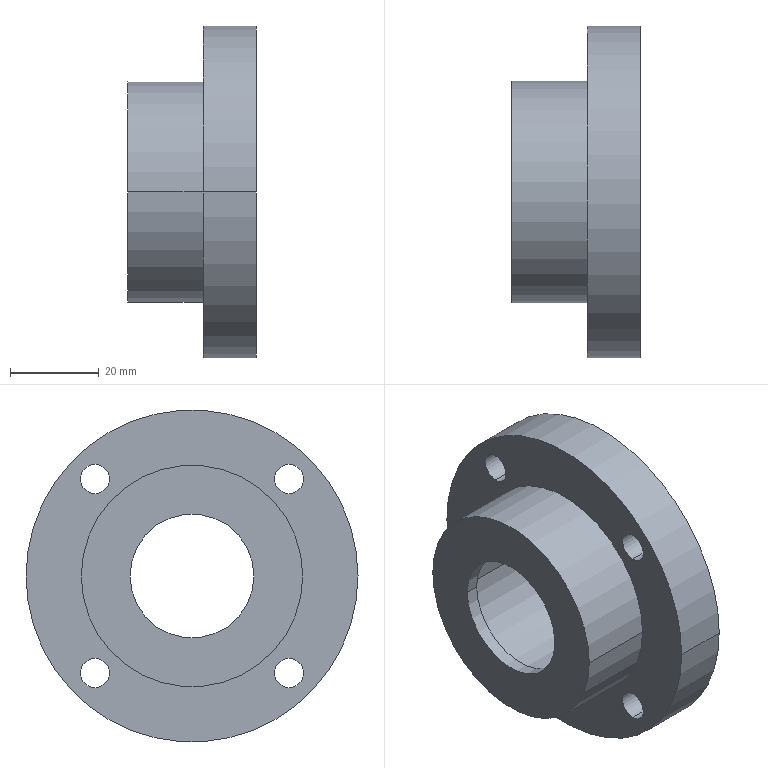Part | SolidWorks | features HoleWzd 2, Chamfer 1, Revolution 1 | 1 solid | 53 faces | box 29 x 75 x 75 mm | volume 54196 mm3 | cylinder 34 | cone 10 | plane 9 | commonest cylinder face diameters 2.5 x8 6.6 x8 11 x8 28 x2 32 x2 48 x2
STEP:
#1=CARTESIAN_POINT('',(-6.5,-16.,0.));
#2=VERTEX_POINT('',#1);
#3=CARTESIAN_POINT('',(-6.5,16.,0.));
#4=VERTEX_POINT('',#3);
#5=CARTESIAN_POINT('',(-6.5,0.,0.));
#6=DIRECTION('',(1.,0.,0.));
#7=DIRECTION('',(0.,1.,0.));
#8=AXIS2_PLACEMENT_3D('',#5,#6,#7);
#9=CIRCLE('',#8,16.);
#10=EDGE_CURVE('',#2,#4,#9,.T.);
#11=ORIENTED_EDGE('',*,*,#10,.F.);
#12=CARTESIAN_POINT('',(-6.,-16.5,0.));
#13=VERTEX_POINT('',#12);
#14=CARTESIAN_POINT('',(-6.5,-16.,0.));
#15=DIRECTION('',(0.7071,-0.7071,0.));
#16=VECTOR('',#15,1000.);
#17=LINE('',#14,#16);
#18=EDGE_CURVE('',#2,#13,#17,.T.);
#19=ORIENTED_EDGE('',*,*,#18,.T.);
#20=CARTESIAN_POINT('',(-6.,16.5,0.));
#21=VERTEX_POINT('',#20);
#22=CARTESIAN_POINT('',(-6.,0.,0.));
#23=DIRECTION('',(-1.,0.,0.));
#24=DIRECTION('',(0.,1.,0.));
#25=AXIS2_PLACEMENT_3D('',#22,#23,#24);
#26=CIRCLE('',#25,16.5);
#27=EDGE_CURVE('',#21,#13,#26,.T.);
#28=ORIENTED_EDGE('',*,*,#27,.F.);
#29=CARTESIAN_POINT('',(-6.5,16.,0.));
#30=DIRECTION('',(0.7071,0.7071,0.));
#31=VECTOR('',#30,1000.);
#32=LINE('',#29,#31);
#33=EDGE_CURVE('',#4,#21,#32,.T.);
#34=ORIENTED_EDGE('',*,*,#33,.F.);
#35=EDGE_LOOP('',(#11,#19,#28,#34));
#36=FACE_OUTER_BOUND('',#35,.T.);
#37=CARTESIAN_POINT('',(-6.5,0.,0.));
#38=DIRECTION('',(1.,0.,0.));
#39=DIRECTION('',(0.,1.,0.));
#40=AXIS2_PLACEMENT_3D('',#37,#38,#39);
#41=CONICAL_SURFACE('',#40,16.,0.7854);
#42=ADVANCED_FACE('',(#36),#41,.F.);
#43=CARTESIAN_POINT('',(-14.5,20.,1.25));
#44=VERTEX_POINT('',#43);
#45=CARTESIAN_POINT('',(-14.5,20.,-1.25));
#46=VERTEX_POINT('',#45);
#47=CARTESIAN_POINT('',(-14.5,20.,0.));
#48=DIRECTION('',(1.,0.,0.));
#49=DIRECTION('',(0.,0.,-1.));
#50=AXIS2_PLACEMENT_3D('',#47,#48,#49);
#51=CIRCLE('',#50,1.25);
#52=EDGE_CURVE('',#44,#46,#51,.T.);
#53=ORIENTED_EDGE('',*,*,#52,.F.);
#54=CARTESIAN_POINT('',(-6.,20.,1.25));
#55=VERTEX_POINT('',#54);
#56=CARTESIAN_POINT('',(-6.,20.,1.25));
#57=DIRECTION('',(1.,0.,0.));
#58=VECTOR('',#57,1000.);
#59=LINE('',#56,#58);
#60=EDGE_CURVE('',#44,#55,#59,.T.);
#61=ORIENTED_EDGE('',*,*,#60,.T.);
#62=CARTESIAN_POINT('',(-6.,20.,-1.25));
#63=VERTEX_POINT('',#62);
#64=CARTESIAN_POINT('',(-6.,20.,0.));
#65=DIRECTION('',(1.,0.,0.));
#66=DIRECTION('',(0.,0.,-1.));
#67=AXIS2_PLACEMENT_3D('',#64,#65,#66);
#68=CIRCLE('',#67,1.25);
#69=EDGE_CURVE('',#55,#63,#68,.T.);
#70=ORIENTED_EDGE('',*,*,#69,.T.);
#71=CARTESIAN_POINT('',(-6.,20.,-1.25));
#72=DIRECTION('',(1.,0.,0.));
#73=VECTOR('',#72,1000.);
#74=LINE('',#71,#73);
#75=EDGE_CURVE('',#46,#63,#74,.T.);
#76=ORIENTED_EDGE('',*,*,#75,.F.);
#77=EDGE_LOOP('',(#53,#61,#70,#76));
#78=FACE_OUTER_BOUND('',#77,.T.);
#79=CARTESIAN_POINT('',(-6.,20.,0.));
#80=DIRECTION('',(1.,0.,0.));
#81=DIRECTION('',(0.,0.,-1.));
#82=AXIS2_PLACEMENT_3D('',#79,#80,#81);
#83=CYLINDRICAL_SURFACE('',#82,1.25);
#84=ADVANCED_FACE('',(#78),#83,.F.);
#85=CARTESIAN_POINT('',(-15.251,20.,0.));
#86=VERTEX_POINT('',#85);
#87=CARTESIAN_POINT('',(-14.5,20.,-1.25));
#88=DIRECTION('',(0.515,0.,-0.8572));
#89=VECTOR('',#88,1000.);
#90=LINE('',#87,#89);
#91=EDGE_CURVE('',#86,#46,#90,.T.);
#92=ORIENTED_EDGE('',*,*,#91,.F.);
#93=CARTESIAN_POINT('',(-14.5,20.,1.25));
#94=DIRECTION('',(0.515,0.,0.8572));
#95=VECTOR('',#94,1000.);
#96=LINE('',#93,#95);
#97=EDGE_CURVE('',#86,#44,#96,.T.);
#98=ORIENTED_EDGE('',*,*,#97,.T.);
#99=ORIENTED_EDGE('',*,*,#52,.T.);
#100=EDGE_LOOP('',(#92,#98,#99));
#101=FACE_OUTER_BOUND('',#100,.T.);
#102=CARTESIAN_POINT('',(-14.5,20.,0.));
#103=DIRECTION('',(1.,0.,0.));
#104=DIRECTION('',(0.,0.,-1.));
#105=AXIS2_PLACEMENT_3D('',#102,#103,#104);
#106=CONICAL_SURFACE('',#105,1.25,1.03);
#107=ADVANCED_FACE('',(#101),#106,.F.);
#108=CARTESIAN_POINT('',(-14.5,0.,21.25));
#109=VERTEX_POINT('',#108);
#110=CARTESIAN_POINT('',(-14.5,0.,18.75));
#111=VERTEX_POINT('',#110);
#112=CARTESIAN_POINT('',(-14.5,0.,20.));
#113=DIRECTION('',(1.,0.,0.));
#114=DIRECTION('',(0.,0.,-1.));
#115=AXIS2_PLACEMENT_3D('',#112,#113,#114);
#116=CIRCLE('',#115,1.25);
#117=EDGE_CURVE('',#109,#111,#116,.T.);
#118=ORIENTED_EDGE('',*,*,#117,.F.);
#119=CARTESIAN_POINT('',(-6.,0.,21.25));
#120=VERTEX_POINT('',#119);
#121=CARTESIAN_POINT('',(-6.,0.,21.25));
#122=DIRECTION('',(1.,0.,0.));
#123=VECTOR('',#122,1000.);
#124=LINE('',#121,#123);
#125=EDGE_CURVE('',#109,#120,#124,.T.);
#126=ORIENTED_EDGE('',*,*,#125,.T.);
#127=CARTESIAN_POINT('',(-6.,0.,18.75));
#128=VERTEX_POINT('',#127);
#129=CARTESIAN_POINT('',(-6.,0.,20.));
#130=DIRECTION('',(1.,0.,0.));
#131=DIRECTION('',(0.,0.,-1.));
#132=AXIS2_PLACEMENT_3D('',#129,#130,#131);
#133=CIRCLE('',#132,1.25);
#134=EDGE_CURVE('',#120,#128,#133,.T.);
#135=ORIENTED_EDGE('',*,*,#134,.T.);
#136=CARTESIAN_POINT('',(-6.,0.,18.75));
#137=DIRECTION('',(1.,0.,0.));
#138=VECTOR('',#137,1000.);
#139=LINE('',#136,#138);
#140=EDGE_CURVE('',#111,#128,#139,.T.);
#141=ORIENTED_EDGE('',*,*,#140,.F.);
#142=EDGE_LOOP('',(#118,#126,#135,#141));
#143=FACE_OUTER_BOUND('',#142,.T.);
#144=CARTESIAN_POINT('',(-6.,0.,20.));
#145=DIRECTION('',(1.,0.,0.));
#146=DIRECTION('',(0.,0.,-1.));
#147=AXIS2_PLACEMENT_3D('',#144,#145,#146);
#148=CYLINDRICAL_SURFACE('',#147,1.25);
#149=ADVANCED_FACE('',(#143),#148,.F.);
#150=CARTESIAN_POINT('',(-15.251,0.,20.));
#151=VERTEX_POINT('',#150);
#152=CARTESIAN_POINT('',(-14.5,0.,18.75));
#153=DIRECTION('',(0.515,0.,-0.8572));
#154=VECTOR('',#153,1000.);
#155=LINE('',#152,#154);
#156=EDGE_CURVE('',#151,#111,#155,.T.);
#157=ORIENTED_EDGE('',*,*,#156,.F.);
#158=CARTESIAN_POINT('',(-14.5,0.,21.25));
#159=DIRECTION('',(0.515,0.,0.8572));
#160=VECTOR('',#159,1000.);
#161=LINE('',#158,#160);
#162=EDGE_CURVE('',#151,#109,#161,.T.);
#163=ORIENTED_EDGE('',*,*,#162,.T.);
#164=ORIENTED_EDGE('',*,*,#117,.T.);
#165=EDGE_LOOP('',(#157,#163,#164));
#166=FACE_OUTER_BOUND('',#165,.T.);
#167=CARTESIAN_POINT('',(-14.5,0.,20.));
#168=DIRECTION('',(1.,0.,0.));
#169=DIRECTION('',(0.,0.,-1.));
#170=AXIS2_PLACEMENT_3D('',#167,#168,#169);
#171=CONICAL_SURFACE('',#170,1.25,1.03);
#172=ADVANCED_FACE('',(#166),#171,.F.);
#173=CARTESIAN_POINT('',(-14.5,-20.,1.25));
#174=VERTEX_POINT('',#173);
#175=CARTESIAN_POINT('',(-14.5,-20.,-1.25));
#176=VERTEX_POINT('',#175);
#177=CARTESIAN_POINT('',(-14.5,-20.,0.));
#178=DIRECTION('',(1.,0.,0.));
#179=DIRECTION('',(0.,0.,-1.));
#180=AXIS2_PLACEMENT_3D('',#177,#178,#179);
#181=CIRCLE('',#180,1.25);
#182=EDGE_CURVE('',#174,#176,#181,.T.);
#183=ORIENTED_EDGE('',*,*,#182,.F.);
#184=CARTESIAN_POINT('',(-6.,-20.,1.25));
#185=VERTEX_POINT('',#184);
#186=CARTESIAN_POINT('',(-6.,-20.,1.25));
#187=DIRECTION('',(1.,0.,0.));
#188=VECTOR('',#187,1000.);
#189=LINE('',#186,#188);
#190=EDGE_CURVE('',#174,#185,#189,.T.);
#191=ORIENTED_EDGE('',*,*,#190,.T.);
#192=CARTESIAN_POINT('',(-6.,-20.,-1.25));
#193=VERTEX_POINT('',#192);
#194=CARTESIAN_POINT('',(-6.,-20.,0.));
#195=DIRECTION('',(1.,0.,0.));
#196=DIRECTION('',(0.,0.,-1.));
#197=AXIS2_PLACEMENT_3D('',#194,#195,#196);
#198=CIRCLE('',#197,1.25);
#199=EDGE_CURVE('',#185,#193,#198,.T.);
#200=ORIENTED_EDGE('',*,*,#199,.T.);
#201=CARTESIAN_POINT('',(-6.,-20.,-1.25));
#202=DIRECTION('',(1.,0.,0.));
#203=VECTOR('',#202,1000.);
#204=LINE('',#201,#203);
#205=EDGE_CURVE('',#176,#193,#204,.T.);
#206=ORIENTED_EDGE('',*,*,#205,.F.);
#207=EDGE_LOOP('',(#183,#191,#200,#206));
#208=FACE_OUTER_BOUND('',#207,.T.);
#209=CARTESIAN_POINT('',(-6.,-20.,0.));
#210=DIRECTION('',(1.,0.,0.));
#211=DIRECTION('',(0.,0.,-1.));
#212=AXIS2_PLACEMENT_3D('',#209,#210,#211);
#213=CYLINDRICAL_SURFACE('',#212,1.25);
#214=ADVANCED_FACE('',(#208),#213,.F.);
#215=CARTESIAN_POINT('',(-15.251,-20.,0.));
#216=VERTEX_POINT('',#215);
#217=CARTESIAN_POINT('',(-14.5,-20.,-1.25));
#218=DIRECTION('',(0.515,0.,-0.8572));
#219=VECTOR('',#218,1000.);
#220=LINE('',#217,#219);
#221=EDGE_CURVE('',#216,#176,#220,.T.);
#222=ORIENTED_EDGE('',*,*,#221,.F.);
#223=CARTESIAN_POINT('',(-14.5,-20.,1.25));
#224=DIRECTION('',(0.515,0.,0.8572));
#225=VECTOR('',#224,1000.);
#226=LINE('',#223,#225);
#227=EDGE_CURVE('',#216,#174,#226,.T.);
#228=ORIENTED_EDGE('',*,*,#227,.T.);
#229=ORIENTED_EDGE('',*,*,#182,.T.);
#230=EDGE_LOOP('',(#222,#228,#229));
#231=FACE_OUTER_BOUND('',#230,.T.);
#232=CARTESIAN_POINT('',(-14.5,-20.,0.));
#233=DIRECTION('',(1.,0.,0.));
#234=DIRECTION('',(0.,0.,-1.));
#235=AXIS2_PLACEMENT_3D('',#232,#233,#234);
#236=CONICAL_SURFACE('',#235,1.25,1.03);
#237=ADVANCED_FACE('',(#231),#236,.F.);
#238=CARTESIAN_POINT('',(-14.5,0.,-18.75));
#239=VERTEX_POINT('',#238);
#240=CARTESIAN_POINT('',(-14.5,0.,-21.25));
#241=VERTEX_POINT('',#240);
#242=CARTESIAN_POINT('',(-14.5,0.,-20.));
#243=DIRECTION('',(1.,0.,0.));
#244=DIRECTION('',(0.,0.,-1.));
#245=AXIS2_PLACEMENT_3D('',#242,#243,#244);
#246=CIRCLE('',#245,1.25);
#247=EDGE_CURVE('',#239,#241,#246,.T.);
#248=ORIENTED_EDGE('',*,*,#247,.F.);
#249=CARTESIAN_POINT('',(-6.,0.,-18.75));
#250=VERTEX_POINT('',#249);
#251=CARTESIAN_POINT('',(-6.,0.,-18.75));
#252=DIRECTION('',(1.,0.,0.));
#253=VECTOR('',#252,1000.);
#254=LINE('',#251,#253);
#255=EDGE_CURVE('',#239,#250,#254,.T.);
#256=ORIENTED_EDGE('',*,*,#255,.T.);
#257=CARTESIAN_POINT('',(-6.,0.,-21.25));
#258=VERTEX_POINT('',#257);
#259=CARTESIAN_POINT('',(-6.,0.,-20.));
#260=DIRECTION('',(1.,0.,0.));
#261=DIRECTION('',(0.,0.,-1.));
#262=AXIS2_PLACEMENT_3D('',#259,#260,#261);
#263=CIRCLE('',#262,1.25);
#264=EDGE_CURVE('',#250,#258,#263,.T.);
#265=ORIENTED_EDGE('',*,*,#264,.T.);
#266=CARTESIAN_POINT('',(-6.,0.,-21.25));
#267=DIRECTION('',(1.,0.,0.));
#268=VECTOR('',#267,1000.);
#269=LINE('',#266,#268);
#270=EDGE_CURVE('',#241,#258,#269,.T.);
#271=ORIENTED_EDGE('',*,*,#270,.F.);
#272=EDGE_LOOP('',(#248,#256,#265,#271));
#273=FACE_OUTER_BOUND('',#272,.T.);
#274=CARTESIAN_POINT('',(-6.,0.,-20.));
#275=DIRECTION('',(1.,0.,0.));
#276=DIRECTION('',(0.,0.,-1.));
#277=AXIS2_PLACEMENT_3D('',#274,#275,#276);
#278=CYLINDRICAL_SURFACE('',#277,1.25);
#279=ADVANCED_FACE('',(#273),#278,.F.);
#280=CARTESIAN_POINT('',(-15.251,0.,-20.));
#281=VERTEX_POINT('',#280);
#282=CARTESIAN_POINT('',(-14.5,0.,-21.25));
#283=DIRECTION('',(0.515,0.,-0.8572));
#284=VECTOR('',#283,1000.);
#285=LINE('',#282,#284);
#286=EDGE_CURVE('',#281,#241,#285,.T.);
#287=ORIENTED_EDGE('',*,*,#286,.F.);
#288=CARTESIAN_POINT('',(-14.5,0.,-18.75));
#289=DIRECTION('',(0.515,0.,0.8572));
#290=VECTOR('',#289,1000.);
#291=LINE('',#288,#290);
#292=EDGE_CURVE('',#281,#239,#291,.T.);
#293=ORIENTED_EDGE('',*,*,#292,.T.);
#294=ORIENTED_EDGE('',*,*,#247,.T.);
#295=EDGE_LOOP('',(#287,#293,#294));
#296=FACE_OUTER_BOUND('',#295,.T.);
#297=CARTESIAN_POINT('',(-14.5,0.,-20.));
#298=DIRECTION('',(1.,0.,0.));
#299=DIRECTION('',(0.,0.,-1.));
#300=AXIS2_PLACEMENT_3D('',#297,#298,#299);
#301=CONICAL_SURFACE('',#300,1.25,1.03);
#302=ADVANCED_FACE('',(#296),#301,.F.);
#303=CARTESIAN_POINT('',(-6.5,21.92,27.42));
#304=VERTEX_POINT('',#303);
#305=CARTESIAN_POINT('',(-6.5,21.92,16.42));
#306=VERTEX_POINT('',#305);
#307=CARTESIAN_POINT('',(-6.5,21.92,21.92));
#308=DIRECTION('',(1.,0.,0.));
#309=DIRECTION('',(0.,0.,-1.));
#310=AXIS2_PLACEMENT_3D('',#307,#308,#309);
#311=CIRCLE('',#310,5.5);
#312=EDGE_CURVE('',#304,#306,#311,.T.);
#313=ORIENTED_EDGE('',*,*,#312,.F.);
#314=CARTESIAN_POINT('',(0.,21.92,27.42));
#315=VERTEX_POINT('',#314);
#316=CARTESIAN_POINT('',(0.,21.92,27.42));
#317=DIRECTION('',(1.,0.,0.));
#318=VECTOR('',#317,1000.);
#319=LINE('',#316,#318);
#320=EDGE_CURVE('',#304,#315,#319,.T.);
#321=ORIENTED_EDGE('',*,*,#320,.T.);
#322=CARTESIAN_POINT('',(0.,21.92,16.42));
#323=VERTEX_POINT('',#322);
#324=CARTESIAN_POINT('',(0.,21.92,21.92));
#325=DIRECTION('',(1.,0.,0.));
#326=DIRECTION('',(0.,0.,-1.));
#327=AXIS2_PLACEMENT_3D('',#324,#325,#326);
#328=CIRCLE('',#327,5.5);
#329=EDGE_CURVE('',#315,#323,#328,.T.);
#330=ORIENTED_EDGE('',*,*,#329,.T.);
#331=CARTESIAN_POINT('',(0.,21.92,16.42));
#332=DIRECTION('',(1.,0.,0.));
#333=VECTOR('',#332,1000.);
#334=LINE('',#331,#333);
#335=EDGE_CURVE('',#306,#323,#334,.T.);
#336=ORIENTED_EDGE('',*,*,#335,.F.);
#337=EDGE_LOOP('',(#313,#321,#330,#336));
#338=FACE_OUTER_BOUND('',#337,.T.);
#339=CARTESIAN_POINT('',(0.,21.92,21.92));
#340=DIRECTION('',(1.,0.,0.));
#341=DIRECTION('',(0.,0.,-1.));
#342=AXIS2_PLACEMENT_3D('',#339,#340,#341);
#343=CYLINDRICAL_SURFACE('',#342,5.5);
#344=ADVANCED_FACE('',(#338),#343,.F.);
#345=CARTESIAN_POINT('',(-12.,21.92,18.62));
#346=VERTEX_POINT('',#345);
#347=CARTESIAN_POINT('',(-12.,21.92,25.22));
#348=VERTEX_POINT('',#347);
#349=CARTESIAN_POINT('',(-12.,21.92,21.92));
#350=DIRECTION('',(-1.,0.,0.));
#351=DIRECTION('',(0.,-1.,0.));
#352=AXIS2_PLACEMENT_3D('',#349,#350,#351);
#353=CIRCLE('',#352,3.3);
#354=EDGE_CURVE('',#346,#348,#353,.T.);
#355=ORIENTED_EDGE('',*,*,#354,.T.);
#356=CARTESIAN_POINT('',(-6.5,21.92,25.22));
#357=VERTEX_POINT('',#356);
#358=CARTESIAN_POINT('',(0.,21.92,25.22));
#359=DIRECTION('',(1.,0.,0.));
#360=VECTOR('',#359,1000.);
#361=LINE('',#358,#360);
#362=EDGE_CURVE('',#348,#357,#361,.T.);
#363=ORIENTED_EDGE('',*,*,#362,.T.);
#364=CARTESIAN_POINT('',(-6.5,21.92,18.62));
#365=VERTEX_POINT('',#364);
#366=CARTESIAN_POINT('',(-6.5,21.92,21.92));
#367=DIRECTION('',(1.,0.,0.));
#368=DIRECTION('',(0.,0.,-1.));
#369=AXIS2_PLACEMENT_3D('',#366,#367,#368);
#370=CIRCLE('',#369,3.3);
#371=EDGE_CURVE('',#357,#365,#370,.T.);
#372=ORIENTED_EDGE('',*,*,#371,.T.);
#373=CARTESIAN_POINT('',(0.,21.92,18.62));
#374=DIRECTION('',(1.,0.,0.));
#375=VECTOR('',#374,1000.);
#376=LINE('',#373,#375);
#377=EDGE_CURVE('',#346,#365,#376,.T.);
#378=ORIENTED_EDGE('',*,*,#377,.F.);
#379=EDGE_LOOP('',(#355,#363,#372,#378));
#380=FACE_OUTER_BOUND('',#379,.T.);
#381=CARTESIAN_POINT('',(0.,21.92,21.92));
#382=DIRECTION('',(1.,0.,0.));
#383=DIRECTION('',(0.,0.,-1.));
#384=AXIS2_PLACEMENT_3D('',#381,#382,#383);
#385=CYLINDRICAL_SURFACE('',#384,3.3);
#386=ADVANCED_FACE('',(#380),#385,.F.);
#387=CARTESIAN_POINT('',(-6.5,21.92,-16.42));
#388=VERTEX_POINT('',#387);
#389=CARTESIAN_POINT('',(-6.5,21.92,-27.42));
#390=VERTEX_POINT('',#389);
#391=CARTESIAN_POINT('',(-6.5,21.92,-21.92));
#392=DIRECTION('',(1.,0.,0.));
#393=DIRECTION('',(0.,0.,-1.));
#394=AXIS2_PLACEMENT_3D('',#391,#392,#393);
#395=CIRCLE('',#394,5.5);
#396=EDGE_CURVE('',#388,#390,#395,.T.);
#397=ORIENTED_EDGE('',*,*,#396,.F.);
#398=CARTESIAN_POINT('',(0.,21.92,-16.42));
#399=VERTEX_POINT('',#398);
#400=CARTESIAN_POINT('',(0.,21.92,-16.42));
#401=DIRECTION('',(1.,0.,0.));
#402=VECTOR('',#401,1000.);
#403=LINE('',#400,#402);
#404=EDGE_CURVE('',#388,#399,#403,.T.);
#405=ORIENTED_EDGE('',*,*,#404,.T.);
#406=CARTESIAN_POINT('',(0.,21.92,-27.42));
#407=VERTEX_POINT('',#406);
#408=CARTESIAN_POINT('',(0.,21.92,-21.92));
#409=DIRECTION('',(1.,0.,0.));
#410=DIRECTION('',(0.,0.,-1.));
#411=AXIS2_PLACEMENT_3D('',#408,#409,#410);
#412=CIRCLE('',#411,5.5);
#413=EDGE_CURVE('',#399,#407,#412,.T.);
#414=ORIENTED_EDGE('',*,*,#413,.T.);
#415=CARTESIAN_POINT('',(0.,21.92,-27.42));
#416=DIRECTION('',(1.,0.,0.));
#417=VECTOR('',#416,1000.);
#418=LINE('',#415,#417);
#419=EDGE_CURVE('',#390,#407,#418,.T.);
#420=ORIENTED_EDGE('',*,*,#419,.F.);
#421=EDGE_LOOP('',(#397,#405,#414,#420));
#422=FACE_OUTER_BOUND('',#421,.T.);
#423=CARTESIAN_POINT('',(0.,21.92,-21.92));
#424=DIRECTION('',(1.,0.,0.));
#425=DIRECTION('',(0.,0.,-1.));
#426=AXIS2_PLACEMENT_3D('',#423,#424,#425);
#427=CYLINDRICAL_SURFACE('',#426,5.5);
#428=ADVANCED_FACE('',(#422),#427,.F.);
#429=CARTESIAN_POINT('',(-12.,21.92,-25.22));
#430=VERTEX_POINT('',#429);
#431=CARTESIAN_POINT('',(-12.,21.92,-18.62));
#432=VERTEX_POINT('',#431);
#433=CARTESIAN_POINT('',(-12.,21.92,-21.92));
#434=DIRECTION('',(-1.,0.,0.));
#435=DIRECTION('',(0.,-1.,0.));
#436=AXIS2_PLACEMENT_3D('',#433,#434,#435);
#437=CIRCLE('',#436,3.3);
#438=EDGE_CURVE('',#430,#432,#437,.T.);
#439=ORIENTED_EDGE('',*,*,#438,.T.);
#440=CARTESIAN_POINT('',(-6.5,21.92,-18.62));
#441=VERTEX_POINT('',#440);
#442=CARTESIAN_POINT('',(0.,21.92,-18.62));
#443=DIRECTION('',(1.,0.,0.));
#444=VECTOR('',#443,1000.);
#445=LINE('',#442,#444);
#446=EDGE_CURVE('',#432,#441,#445,.T.);
#447=ORIENTED_EDGE('',*,*,#446,.T.);
#448=CARTESIAN_POINT('',(-6.5,21.92,-25.22));
#449=VERTEX_POINT('',#448);
#450=CARTESIAN_POINT('',(-6.5,21.92,-21.92));
#451=DIRECTION('',(1.,0.,0.));
#452=DIRECTION('',(0.,0.,-1.));
#453=AXIS2_PLACEMENT_3D('',#450,#451,#452);
#454=CIRCLE('',#453,3.3);
#455=EDGE_CURVE('',#441,#449,#454,.T.);
#456=ORIENTED_EDGE('',*,*,#455,.T.);
#457=CARTESIAN_POINT('',(0.,21.92,-25.22));
#458=DIRECTION('',(1.,0.,0.));
#459=VECTOR('',#458,1000.);
#460=LINE('',#457,#459);
#461=EDGE_CURVE('',#430,#449,#460,.T.);
#462=ORIENTED_EDGE('',*,*,#461,.F.);
#463=EDGE_LOOP('',(#439,#447,#456,#462));
#464=FACE_OUTER_BOUND('',#463,.T.);
#465=CARTESIAN_POINT('',(0.,21.92,-21.92));
#466=DIRECTION('',(1.,0.,0.));
#467=DIRECTION('',(0.,0.,-1.));
#468=AXIS2_PLACEMENT_3D('',#465,#466,#467);
#469=CYLINDRICAL_SURFACE('',#468,3.3);
#470=ADVANCED_FACE('',(#464),#469,.F.);
#471=CARTESIAN_POINT('',(-6.5,-21.92,-16.42));
#472=VERTEX_POINT('',#471);
#473=CARTESIAN_POINT('',(-6.5,-21.92,-27.42));
#474=VERTEX_POINT('',#473);
#475=CARTESIAN_POINT('',(-6.5,-21.92,-21.92));
#476=DIRECTION('',(1.,0.,0.));
#477=DIRECTION('',(0.,0.,-1.));
#478=AXIS2_PLACEMENT_3D('',#475,#476,#477);
#479=CIRCLE('',#478,5.5);
#480=EDGE_CURVE('',#472,#474,#479,.T.);
#481=ORIENTED_EDGE('',*,*,#480,.F.);
#482=CARTESIAN_POINT('',(0.,-21.92,-16.42));
#483=VERTEX_POINT('',#482);
#484=CARTESIAN_POINT('',(0.,-21.92,-16.42));
#485=DIRECTION('',(1.,0.,0.));
#486=VECTOR('',#485,1000.);
#487=LINE('',#484,#486);
#488=EDGE_CURVE('',#472,#483,#487,.T.);
#489=ORIENTED_EDGE('',*,*,#488,.T.);
#490=CARTESIAN_POINT('',(0.,-21.92,-27.42));
#491=VERTEX_POINT('',#490);
#492=CARTESIAN_POINT('',(0.,-21.92,-21.92));
#493=DIRECTION('',(1.,0.,0.));
#494=DIRECTION('',(0.,0.,-1.));
#495=AXIS2_PLACEMENT_3D('',#492,#493,#494);
#496=CIRCLE('',#495,5.5);
#497=EDGE_CURVE('',#483,#491,#496,.T.);
#498=ORIENTED_EDGE('',*,*,#497,.T.);
#499=CARTESIAN_POINT('',(0.,-21.92,-27.42));
#500=DIRECTION('',(1.,0.,0.));
#501=VECTOR('',#500,1000.);
#502=LINE('',#499,#501);
#503=EDGE_CURVE('',#474,#491,#502,.T.);
#504=ORIENTED_EDGE('',*,*,#503,.F.);
#505=EDGE_LOOP('',(#481,#489,#498,#504));
#506=FACE_OUTER_BOUND('',#505,.T.);
#507=CARTESIAN_POINT('',(0.,-21.92,-21.92));
#508=DIRECTION('',(1.,0.,0.));
#509=DIRECTION('',(0.,0.,-1.));
#510=AXIS2_PLACEMENT_3D('',#507,#508,#509);
#511=CYLINDRICAL_SURFACE('',#510,5.5);
#512=ADVANCED_FACE('',(#506),#511,.F.);
#513=CARTESIAN_POINT('',(-12.,-21.92,-25.22));
#514=VERTEX_POINT('',#513);
#515=CARTESIAN_POINT('',(-12.,-21.92,-18.62));
#516=VERTEX_POINT('',#515);
#517=CARTESIAN_POINT('',(-12.,-21.92,-21.92));
#518=DIRECTION('',(-1.,0.,0.));
#519=DIRECTION('',(0.,-1.,0.));
#520=AXIS2_PLACEMENT_3D('',#517,#518,#519);
#521=CIRCLE('',#520,3.3);
#522=EDGE_CURVE('',#514,#516,#521,.T.);
#523=ORIENTED_EDGE('',*,*,#522,.T.);
#524=CARTESIAN_POINT('',(-6.5,-21.92,-18.62));
#525=VERTEX_POINT('',#524);
#526=CARTESIAN_POINT('',(0.,-21.92,-18.62));
#527=DIRECTION('',(1.,0.,0.));
#528=VECTOR('',#527,1000.);
#529=LINE('',#526,#528);
#530=EDGE_CURVE('',#516,#525,#529,.T.);
#531=ORIENTED_EDGE('',*,*,#530,.T.);
#532=CARTESIAN_POINT('',(-6.5,-21.92,-25.22));
#533=VERTEX_POINT('',#532);
#534=CARTESIAN_POINT('',(-6.5,-21.92,-21.92));
#535=DIRECTION('',(1.,0.,0.));
#536=DIRECTION('',(0.,0.,-1.));
#537=AXIS2_PLACEMENT_3D('',#534,#535,#536);
#538=CIRCLE('',#537,3.3);
#539=EDGE_CURVE('',#525,#533,#538,.T.);
#540=ORIENTED_EDGE('',*,*,#539,.T.);
#541=CARTESIAN_POINT('',(0.,-21.92,-25.22));
#542=DIRECTION('',(1.,0.,0.));
#543=VECTOR('',#542,1000.);
#544=LINE('',#541,#543);
#545=EDGE_CURVE('',#514,#533,#544,.T.);
#546=ORIENTED_EDGE('',*,*,#545,.F.);
#547=EDGE_LOOP('',(#523,#531,#540,#546));
#548=FACE_OUTER_BOUND('',#547,.T.);
#549=CARTESIAN_POINT('',(0.,-21.92,-21.92));
#550=DIRECTION('',(1.,0.,0.));
#551=DIRECTION('',(0.,0.,-1.));
#552=AXIS2_PLACEMENT_3D('',#549,#550,#551);
#553=CYLINDRICAL_SURFACE('',#552,3.3);
#554=ADVANCED_FACE('',(#548),#553,.F.);
#555=CARTESIAN_POINT('',(-6.5,-21.92,27.42));
#556=VERTEX_POINT('',#555);
#557=CARTESIAN_POINT('',(-6.5,-21.92,16.42));
#558=VERTEX_POINT('',#557);
#559=CARTESIAN_POINT('',(-6.5,-21.92,21.92));
#560=DIRECTION('',(1.,0.,0.));
#561=DIRECTION('',(0.,0.,-1.));
#562=AXIS2_PLACEMENT_3D('',#559,#560,#561);
#563=CIRCLE('',#562,5.5);
#564=EDGE_CURVE('',#556,#558,#563,.T.);
#565=ORIENTED_EDGE('',*,*,#564,.F.);
#566=CARTESIAN_POINT('',(0.,-21.92,27.42));
#567=VERTEX_POINT('',#566);
#568=CARTESIAN_POINT('',(0.,-21.92,27.42));
#569=DIRECTION('',(1.,0.,0.));
#570=VECTOR('',#569,1000.);
#571=LINE('',#568,#570);
#572=EDGE_CURVE('',#556,#567,#571,.T.);
#573=ORIENTED_EDGE('',*,*,#572,.T.);
#574=CARTESIAN_POINT('',(0.,-21.92,16.42));
#575=VERTEX_POINT('',#574);
#576=CARTESIAN_POINT('',(0.,-21.92,21.92));
#577=DIRECTION('',(1.,0.,0.));
#578=DIRECTION('',(0.,0.,-1.));
#579=AXIS2_PLACEMENT_3D('',#576,#577,#578);
#580=CIRCLE('',#579,5.5);
#581=EDGE_CURVE('',#567,#575,#580,.T.);
#582=ORIENTED_EDGE('',*,*,#581,.T.);
#583=CARTESIAN_POINT('',(0.,-21.92,16.42));
#584=DIRECTION('',(1.,0.,0.));
#585=VECTOR('',#584,1000.);
#586=LINE('',#583,#585);
#587=EDGE_CURVE('',#558,#575,#586,.T.);
#588=ORIENTED_EDGE('',*,*,#587,.F.);
#589=EDGE_LOOP('',(#565,#573,#582,#588));
#590=FACE_OUTER_BOUND('',#589,.T.);
#591=CARTESIAN_POINT('',(0.,-21.92,21.92));
#592=DIRECTION('',(1.,0.,0.));
#593=DIRECTION('',(0.,0.,-1.));
#594=AXIS2_PLACEMENT_3D('',#591,#592,#593);
#595=CYLINDRICAL_SURFACE('',#594,5.5);
#596=ADVANCED_FACE('',(#590),#595,.F.);
#597=CARTESIAN_POINT('',(-12.,-21.92,18.62));
#598=VERTEX_POINT('',#597);
#599=CARTESIAN_POINT('',(-12.,-21.92,25.22));
#600=VERTEX_POINT('',#599);
#601=CARTESIAN_POINT('',(-12.,-21.92,21.92));
#602=DIRECTION('',(-1.,0.,0.));
#603=DIRECTION('',(0.,-1.,0.));
#604=AXIS2_PLACEMENT_3D('',#601,#602,#603);
#605=CIRCLE('',#604,3.3);
#606=EDGE_CURVE('',#598,#600,#605,.T.);
#607=ORIENTED_EDGE('',*,*,#606,.T.);
#608=CARTESIAN_POINT('',(-6.5,-21.92,25.22));
#609=VERTEX_POINT('',#608);
#610=CARTESIAN_POINT('',(0.,-21.92,25.22));
#611=DIRECTION('',(1.,0.,0.));
#612=VECTOR('',#611,1000.);
#613=LINE('',#610,#612);
#614=EDGE_CURVE('',#600,#609,#613,.T.);
#615=ORIENTED_EDGE('',*,*,#614,.T.);
#616=CARTESIAN_POINT('',(-6.5,-21.92,18.62));
#617=VERTEX_POINT('',#616);
#618=CARTESIAN_POINT('',(-6.5,-21.92,21.92));
#619=DIRECTION('',(1.,0.,0.));
#620=DIRECTION('',(0.,0.,-1.));
#621=AXIS2_PLACEMENT_3D('',#618,#619,#620);
#622=CIRCLE('',#621,3.3);
#623=EDGE_CURVE('',#609,#617,#622,.T.);
#624=ORIENTED_EDGE('',*,*,#623,.T.);
#625=CARTESIAN_POINT('',(0.,-21.92,18.62));
#626=DIRECTION('',(1.,0.,0.));
#627=VECTOR('',#626,1000.);
#628=LINE('',#625,#627);
#629=EDGE_CURVE('',#598,#617,#628,.T.);
#630=ORIENTED_EDGE('',*,*,#629,.F.);
#631=EDGE_LOOP('',(#607,#615,#624,#630));
#632=FACE_OUTER_BOUND('',#631,.T.);
#633=CARTESIAN_POINT('',(0.,-21.92,21.92));
#634=DIRECTION('',(1.,0.,0.));
#635=DIRECTION('',(0.,0.,-1.));
#636=AXIS2_PLACEMENT_3D('',#633,#634,#635);
#637=CYLINDRICAL_SURFACE('',#636,3.3);
#638=ADVANCED_FACE('',(#632),#637,.F.);
#639=CARTESIAN_POINT('',(-12.,37.5,0.));
#640=VERTEX_POINT('',#639);
#641=CARTESIAN_POINT('',(-12.,-37.5,0.));
#642=VERTEX_POINT('',#641);
#643=CARTESIAN_POINT('',(-12.,0.,0.));
#644=DIRECTION('',(1.,0.,0.));
#645=DIRECTION('',(0.,1.,0.));
#646=AXIS2_PLACEMENT_3D('',#643,#644,#645);
#647=CIRCLE('',#646,37.5);
#648=EDGE_CURVE('',#640,#642,#647,.T.);
#649=ORIENTED_EDGE('',*,*,#648,.T.);
#650=CARTESIAN_POINT('',(0.,-37.5,0.));
#651=VERTEX_POINT('',#650);
#652=CARTESIAN_POINT('',(0.,-37.5,0.));
#653=DIRECTION('',(1.,0.,0.));
#654=VECTOR('',#653,1000.);
#655=LINE('',#652,#654);
#656=EDGE_CURVE('',#642,#651,#655,.T.);
#657=ORIENTED_EDGE('',*,*,#656,.T.);
#658=CARTESIAN_POINT('',(0.,37.5,0.));
#659=VERTEX_POINT('',#658);
#660=CARTESIAN_POINT('',(0.,0.,0.));
#661=DIRECTION('',(1.,0.,0.));
#662=DIRECTION('',(0.,1.,0.));
#663=AXIS2_PLACEMENT_3D('',#660,#661,#662);
#664=CIRCLE('',#663,37.5);
#665=EDGE_CURVE('',#659,#651,#664,.T.);
#666=ORIENTED_EDGE('',*,*,#665,.F.);
#667=CARTESIAN_POINT('',(0.,37.5,0.));
#668=DIRECTION('',(1.,0.,0.));
#669=VECTOR('',#668,1000.);
#670=LINE('',#667,#669);
#671=EDGE_CURVE('',#640,#659,#670,.T.);
#672=ORIENTED_EDGE('',*,*,#671,.F.);
#673=EDGE_LOOP('',(#649,#657,#666,#672));
#674=FACE_OUTER_BOUND('',#673,.T.);
#675=CARTESIAN_POINT('',(0.,0.,0.));
#676=DIRECTION('',(1.,0.,0.));
#677=DIRECTION('',(0.,1.,0.));
#678=AXIS2_PLACEMENT_3D('',#675,#676,#677);
#679=CYLINDRICAL_SURFACE('',#678,37.5);
#680=ADVANCED_FACE('',(#674),#679,.T.);
#681=CARTESIAN_POINT('',(-29.,25.,0.));
#682=VERTEX_POINT('',#681);
#683=CARTESIAN_POINT('',(-29.,-25.,0.));
#684=VERTEX_POINT('',#683);
#685=CARTESIAN_POINT('',(-29.,0.,0.));
#686=DIRECTION('',(1.,0.,0.));
#687=DIRECTION('',(0.,1.,0.));
#688=AXIS2_PLACEMENT_3D('',#685,#686,#687);
#689=CIRCLE('',#688,25.);
#690=EDGE_CURVE('',#682,#684,#689,.T.);
#691=ORIENTED_EDGE('',*,*,#690,.T.);
#692=CARTESIAN_POINT('',(-12.,-25.,0.));
#693=VERTEX_POINT('',#692);
#694=CARTESIAN_POINT('',(0.,-25.,0.));
#695=DIRECTION('',(1.,0.,0.));
#696=VECTOR('',#695,1000.);
#697=LINE('',#694,#696);
#698=EDGE_CURVE('',#684,#693,#697,.T.);
#699=ORIENTED_EDGE('',*,*,#698,.T.);
#700=CARTESIAN_POINT('',(-12.,25.,0.));
#701=VERTEX_POINT('',#700);
#702=CARTESIAN_POINT('',(-12.,0.,0.));
#703=DIRECTION('',(1.,0.,0.));
#704=DIRECTION('',(0.,1.,0.));
#705=AXIS2_PLACEMENT_3D('',#702,#703,#704);
#706=CIRCLE('',#705,25.);
#707=EDGE_CURVE('',#701,#693,#706,.T.);
#708=ORIENTED_EDGE('',*,*,#707,.F.);
#709=CARTESIAN_POINT('',(0.,25.,0.));
#710=DIRECTION('',(1.,0.,0.));
#711=VECTOR('',#710,1000.);
#712=LINE('',#709,#711);
#713=EDGE_CURVE('',#682,#701,#712,.T.);
#714=ORIENTED_EDGE('',*,*,#713,.F.);
#715=EDGE_LOOP('',(#691,#699,#708,#714));
#716=FACE_OUTER_BOUND('',#715,.T.);
#717=CARTESIAN_POINT('',(0.,0.,0.));
#718=DIRECTION('',(1.,0.,0.));
#719=DIRECTION('',(0.,1.,0.));
#720=AXIS2_PLACEMENT_3D('',#717,#718,#719);
#721=CYLINDRICAL_SURFACE('',#720,25.);
#722=ADVANCED_FACE('',(#716),#721,.T.);
#723=CARTESIAN_POINT('',(-29.,-14.,0.));
#724=VERTEX_POINT('',#723);
#725=CARTESIAN_POINT('',(-29.,14.,0.));
#726=VERTEX_POINT('',#725);
#727=CARTESIAN_POINT('',(-29.,0.,0.));
#728=DIRECTION('',(1.,0.,0.));
#729=DIRECTION('',(0.,1.,0.));
#730=AXIS2_PLACEMENT_3D('',#727,#728,#729);
#731=CIRCLE('',#730,14.);
#732=EDGE_CURVE('',#724,#726,#731,.T.);
#733=ORIENTED_EDGE('',*,*,#732,.F.);
#734=CARTESIAN_POINT('',(-26.,-14.,0.));
#735=VERTEX_POINT('',#734);
#736=CARTESIAN_POINT('',(0.,-14.,0.));
#737=DIRECTION('',(1.,0.,0.));
#738=VECTOR('',#737,1000.);
#739=LINE('',#736,#738);
#740=EDGE_CURVE('',#724,#735,#739,.T.);
#741=ORIENTED_EDGE('',*,*,#740,.T.);
#742=CARTESIAN_POINT('',(-26.,14.,0.));
#743=VERTEX_POINT('',#742);
#744=CARTESIAN_POINT('',(-26.,0.,0.));
#745=DIRECTION('',(1.,0.,0.));
#746=DIRECTION('',(0.,1.,0.));
#747=AXIS2_PLACEMENT_3D('',#744,#745,#746);
#748=CIRCLE('',#747,14.);
#749=EDGE_CURVE('',#735,#743,#748,.T.);
#750=ORIENTED_EDGE('',*,*,#749,.T.);
#751=CARTESIAN_POINT('',(0.,14.,0.));
#752=DIRECTION('',(1.,0.,0.));
#753=VECTOR('',#752,1000.);
#754=LINE('',#751,#753);
#755=EDGE_CURVE('',#726,#743,#754,.T.);
#756=ORIENTED_EDGE('',*,*,#755,.F.);
#757=EDGE_LOOP('',(#733,#741,#750,#756));
#758=FACE_OUTER_BOUND('',#757,.T.);
#759=CARTESIAN_POINT('',(0.,0.,0.));
#760=DIRECTION('',(1.,0.,0.));
#761=DIRECTION('',(0.,1.,0.));
#762=AXIS2_PLACEMENT_3D('',#759,#760,#761);
#763=CYLINDRICAL_SURFACE('',#762,14.);
#764=ADVANCED_FACE('',(#758),#763,.F.);
#765=CARTESIAN_POINT('',(-26.,-16.,0.));
#766=VERTEX_POINT('',#765);
#767=CARTESIAN_POINT('',(-26.,16.,0.));
#768=VERTEX_POINT('',#767);
#769=CARTESIAN_POINT('',(-26.,0.,0.));
#770=DIRECTION('',(1.,0.,0.));
#771=DIRECTION('',(0.,1.,0.));
#772=AXIS2_PLACEMENT_3D('',#769,#770,#771);
#773=CIRCLE('',#772,16.);
#774=EDGE_CURVE('',#766,#768,#773,.T.);
#775=ORIENTED_EDGE('',*,*,#774,.F.);
#776=CARTESIAN_POINT('',(0.,-16.,0.));
#777=DIRECTION('',(1.,0.,0.));
#778=VECTOR('',#777,1000.);
#779=LINE('',#776,#778);
#780=EDGE_CURVE('',#766,#2,#779,.T.);
#781=ORIENTED_EDGE('',*,*,#780,.T.);
#782=ORIENTED_EDGE('',*,*,#10,.T.);
#783=CARTESIAN_POINT('',(0.,16.,0.));
#784=DIRECTION('',(1.,0.,0.));
#785=VECTOR('',#784,1000.);
#786=LINE('',#783,#785);
#787=EDGE_CURVE('',#768,#4,#786,.T.);
#788=ORIENTED_EDGE('',*,*,#787,.F.);
#789=EDGE_LOOP('',(#775,#781,#782,#788));
#790=FACE_OUTER_BOUND('',#789,.T.);
#791=CARTESIAN_POINT('',(0.,0.,0.));
#792=DIRECTION('',(1.,0.,0.));
#793=DIRECTION('',(0.,1.,0.));
#794=AXIS2_PLACEMENT_3D('',#791,#792,#793);
#795=CYLINDRICAL_SURFACE('',#794,16.);
#796=ADVANCED_FACE('',(#790),#795,.F.);
#797=CARTESIAN_POINT('',(-6.,-24.,0.));
#798=VERTEX_POINT('',#797);
#799=CARTESIAN_POINT('',(-6.,24.,0.));
#800=VERTEX_POINT('',#799);
#801=CARTESIAN_POINT('',(-6.,0.,0.));
#802=DIRECTION('',(1.,0.,0.));
#803=DIRECTION('',(0.,1.,0.));
#804=AXIS2_PLACEMENT_3D('',#801,#802,#803);
#805=CIRCLE('',#804,24.);
#806=EDGE_CURVE('',#798,#800,#805,.T.);
#807=ORIENTED_EDGE('',*,*,#806,.F.);
#808=CARTESIAN_POINT('',(0.,-24.,0.));
#809=VERTEX_POINT('',#808);
#810=CARTESIAN_POINT('',(0.,-24.,0.));
#811=DIRECTION('',(1.,0.,0.));
#812=VECTOR('',#811,1000.);
#813=LINE('',#810,#812);
#814=EDGE_CURVE('',#798,#809,#813,.T.);
#815=ORIENTED_EDGE('',*,*,#814,.T.);
#816=CARTESIAN_POINT('',(0.,24.,0.));
#817=VERTEX_POINT('',#816);
#818=CARTESIAN_POINT('',(0.,0.,0.));
#819=DIRECTION('',(1.,0.,0.));
#820=DIRECTION('',(0.,1.,0.));
#821=AXIS2_PLACEMENT_3D('',#818,#819,#820);
#822=CIRCLE('',#821,24.);
#823=EDGE_CURVE('',#809,#817,#822,.T.);
#824=ORIENTED_EDGE('',*,*,#823,.T.);
#825=CARTESIAN_POINT('',(0.,24.,0.));
#826=DIRECTION('',(1.,0.,0.));
#827=VECTOR('',#826,1000.);
#828=LINE('',#825,#827);
#829=EDGE_CURVE('',#800,#817,#828,.T.);
#830=ORIENTED_EDGE('',*,*,#829,.F.);
#831=EDGE_LOOP('',(#807,#815,#824,#830));
#832=FACE_OUTER_BOUND('',#831,.T.);
#833=CARTESIAN_POINT('',(0.,0.,0.));
#834=DIRECTION('',(1.,0.,0.));
#835=DIRECTION('',(0.,1.,0.));
#836=AXIS2_PLACEMENT_3D('',#833,#834,#835);
#837=CYLINDRICAL_SURFACE('',#836,24.);
#838=ADVANCED_FACE('',(#832),#837,.F.);
#839=CARTESIAN_POINT('',(0.,21.92,21.92));
#840=DIRECTION('',(1.,0.,0.));
#841=DIRECTION('',(0.,0.,-1.));
#842=AXIS2_PLACEMENT_3D('',#839,#840,#841);
#843=CIRCLE('',#842,5.5);
#844=EDGE_CURVE('',#323,#315,#843,.T.);
#845=ORIENTED_EDGE('',*,*,#844,.F.);
#846=ORIENTED_EDGE('',*,*,#329,.F.);
#847=EDGE_LOOP('',(#845,#846));
#848=FACE_BOUND('',#847,.T.);
#849=CARTESIAN_POINT('',(0.,21.92,-21.92));
#850=DIRECTION('',(1.,0.,0.));
#851=DIRECTION('',(0.,0.,-1.));
#852=AXIS2_PLACEMENT_3D('',#849,#850,#851);
#853=CIRCLE('',#852,5.5);
#854=EDGE_CURVE('',#407,#399,#853,.T.);
#855=ORIENTED_EDGE('',*,*,#854,.F.);
#856=ORIENTED_EDGE('',*,*,#413,.F.);
#857=EDGE_LOOP('',(#855,#856));
#858=FACE_BOUND('',#857,.T.);
#859=CARTESIAN_POINT('',(0.,-21.92,-21.92));
#860=DIRECTION('',(1.,0.,0.));
#861=DIRECTION('',(0.,0.,-1.));
#862=AXIS2_PLACEMENT_3D('',#859,#860,#861);
#863=CIRCLE('',#862,5.5);
#864=EDGE_CURVE('',#491,#483,#863,.T.);
#865=ORIENTED_EDGE('',*,*,#864,.F.);
#866=ORIENTED_EDGE('',*,*,#497,.F.);
#867=EDGE_LOOP('',(#865,#866));
#868=FACE_BOUND('',#867,.T.);
#869=CARTESIAN_POINT('',(0.,-21.92,21.92));
#870=DIRECTION('',(1.,0.,0.));
#871=DIRECTION('',(0.,0.,-1.));
#872=AXIS2_PLACEMENT_3D('',#869,#870,#871);
#873=CIRCLE('',#872,5.5);
#874=EDGE_CURVE('',#575,#567,#873,.T.);
#875=ORIENTED_EDGE('',*,*,#874,.F.);
#876=ORIENTED_EDGE('',*,*,#581,.F.);
#877=EDGE_LOOP('',(#875,#876));
#878=FACE_BOUND('',#877,.T.);
#879=ORIENTED_EDGE('',*,*,#665,.T.);
#880=CARTESIAN_POINT('',(0.,0.,0.));
#881=DIRECTION('',(1.,0.,0.));
#882=DIRECTION('',(0.,1.,0.));
#883=AXIS2_PLACEMENT_3D('',#880,#881,#882);
#884=CIRCLE('',#883,37.5);
#885=EDGE_CURVE('',#651,#659,#884,.T.);
#886=ORIENTED_EDGE('',*,*,#885,.T.);
#887=EDGE_LOOP('',(#879,#886));
#888=FACE_OUTER_BOUND('',#887,.T.);
#889=CARTESIAN_POINT('',(0.,0.,0.));
#890=DIRECTION('',(1.,0.,0.));
#891=DIRECTION('',(0.,1.,0.));
#892=AXIS2_PLACEMENT_3D('',#889,#890,#891);
#893=CIRCLE('',#892,24.);
#894=EDGE_CURVE('',#817,#809,#893,.T.);
#895=ORIENTED_EDGE('',*,*,#894,.F.);
#896=ORIENTED_EDGE('',*,*,#823,.F.);
#897=EDGE_LOOP('',(#895,#896));
#898=FACE_BOUND('',#897,.T.);
#899=CARTESIAN_POINT('',(0.,37.5,0.));
#900=DIRECTION('',(1.,0.,0.));
#901=DIRECTION('',(0.,1.,0.));
#902=AXIS2_PLACEMENT_3D('',#899,#900,#901);
#903=PLANE('',#902);
#904=ADVANCED_FACE('',(#848,#858,#868,#878,#888,#898),#903,.T.);
#905=ORIENTED_EDGE('',*,*,#814,.F.);
#906=CARTESIAN_POINT('',(-6.,0.,0.));
#907=DIRECTION('',(1.,0.,0.));
#908=DIRECTION('',(0.,1.,0.));
#909=AXIS2_PLACEMENT_3D('',#906,#907,#908);
#910=CIRCLE('',#909,24.);
#911=EDGE_CURVE('',#800,#798,#910,.T.);
#912=ORIENTED_EDGE('',*,*,#911,.F.);
#913=ORIENTED_EDGE('',*,*,#829,.T.);
#914=ORIENTED_EDGE('',*,*,#894,.T.);
#915=EDGE_LOOP('',(#905,#912,#913,#914));
#916=FACE_OUTER_BOUND('',#915,.T.);
#917=CARTESIAN_POINT('',(0.,0.,0.));
#918=DIRECTION('',(1.,0.,0.));
#919=DIRECTION('',(0.,1.,0.));
#920=AXIS2_PLACEMENT_3D('',#917,#918,#919);
#921=CYLINDRICAL_SURFACE('',#920,24.);
#922=ADVANCED_FACE('',(#916),#921,.F.);
#923=ORIENTED_EDGE('',*,*,#27,.T.);
#924=CARTESIAN_POINT('',(-6.,0.,0.));
#925=DIRECTION('',(-1.,0.,0.));
#926=DIRECTION('',(0.,1.,0.));
#927=AXIS2_PLACEMENT_3D('',#924,#925,#926);
#928=CIRCLE('',#927,16.5);
#929=EDGE_CURVE('',#13,#21,#928,.T.);
#930=ORIENTED_EDGE('',*,*,#929,.T.);
#931=EDGE_LOOP('',(#923,#930));
#932=FACE_BOUND('',#931,.T.);
#933=CARTESIAN_POINT('',(-6.,20.,0.));
#934=DIRECTION('',(1.,0.,0.));
#935=DIRECTION('',(0.,0.,-1.));
#936=AXIS2_PLACEMENT_3D('',#933,#934,#935);
#937=CIRCLE('',#936,1.25);
#938=EDGE_CURVE('',#63,#55,#937,.T.);
#939=ORIENTED_EDGE('',*,*,#938,.F.);
#940=ORIENTED_EDGE('',*,*,#69,.F.);
#941=EDGE_LOOP('',(#939,#940));
#942=FACE_BOUND('',#941,.T.);
#943=CARTESIAN_POINT('',(-6.,0.,20.));
#944=DIRECTION('',(1.,0.,0.));
#945=DIRECTION('',(0.,0.,-1.));
#946=AXIS2_PLACEMENT_3D('',#943,#944,#945);
#947=CIRCLE('',#946,1.25);
#948=EDGE_CURVE('',#128,#120,#947,.T.);
#949=ORIENTED_EDGE('',*,*,#948,.F.);
#950=ORIENTED_EDGE('',*,*,#134,.F.);
#951=EDGE_LOOP('',(#949,#950));
#952=FACE_BOUND('',#951,.T.);
#953=CARTESIAN_POINT('',(-6.,-20.,0.));
#954=DIRECTION('',(1.,0.,0.));
#955=DIRECTION('',(0.,0.,-1.));
#956=AXIS2_PLACEMENT_3D('',#953,#954,#955);
#957=CIRCLE('',#956,1.25);
#958=EDGE_CURVE('',#193,#185,#957,.T.);
#959=ORIENTED_EDGE('',*,*,#958,.F.);
#960=ORIENTED_EDGE('',*,*,#199,.F.);
#961=EDGE_LOOP('',(#959,#960));
#962=FACE_BOUND('',#961,.T.);
#963=CARTESIAN_POINT('',(-6.,0.,-20.));
#964=DIRECTION('',(1.,0.,0.));
#965=DIRECTION('',(0.,0.,-1.));
#966=AXIS2_PLACEMENT_3D('',#963,#964,#965);
#967=CIRCLE('',#966,1.25);
#968=EDGE_CURVE('',#258,#250,#967,.T.);
#969=ORIENTED_EDGE('',*,*,#968,.F.);
#970=ORIENTED_EDGE('',*,*,#264,.F.);
#971=EDGE_LOOP('',(#969,#970));
#972=FACE_BOUND('',#971,.T.);
#973=ORIENTED_EDGE('',*,*,#911,.T.);
#974=ORIENTED_EDGE('',*,*,#806,.T.);
#975=EDGE_LOOP('',(#973,#974));
#976=FACE_OUTER_BOUND('',#975,.T.);
#977=CARTESIAN_POINT('',(-6.,24.,0.));
#978=DIRECTION('',(1.,0.,0.));
#979=DIRECTION('',(0.,1.,0.));
#980=AXIS2_PLACEMENT_3D('',#977,#978,#979);
#981=PLANE('',#980);
#982=ADVANCED_FACE('',(#932,#942,#952,#962,#972,#976),#981,.T.);
#983=ORIENTED_EDGE('',*,*,#780,.F.);
#984=CARTESIAN_POINT('',(-26.,0.,0.));
#985=DIRECTION('',(1.,0.,0.));
#986=DIRECTION('',(0.,1.,0.));
#987=AXIS2_PLACEMENT_3D('',#984,#985,#986);
#988=CIRCLE('',#987,16.);
#989=EDGE_CURVE('',#768,#766,#988,.T.);
#990=ORIENTED_EDGE('',*,*,#989,.F.);
#991=ORIENTED_EDGE('',*,*,#787,.T.);
#992=CARTESIAN_POINT('',(-6.5,0.,0.));
#993=DIRECTION('',(1.,0.,0.));
#994=DIRECTION('',(0.,1.,0.));
#995=AXIS2_PLACEMENT_3D('',#992,#993,#994);
#996=CIRCLE('',#995,16.);
#997=EDGE_CURVE('',#4,#2,#996,.T.);
#998=ORIENTED_EDGE('',*,*,#997,.T.);
#999=EDGE_LOOP('',(#983,#990,#991,#998));
#1000=FACE_OUTER_BOUND('',#999,.T.);
#1001=CARTESIAN_POINT('',(0.,0.,0.));
#1002=DIRECTION('',(1.,0.,0.));
#1003=DIRECTION('',(0.,1.,0.));
#1004=AXIS2_PLACEMENT_3D('',#1001,#1002,#1003);
#1005=CYLINDRICAL_SURFACE('',#1004,16.);
#1006=ADVANCED_FACE('',(#1000),#1005,.F.);
#1007=ORIENTED_EDGE('',*,*,#989,.T.);
#1008=ORIENTED_EDGE('',*,*,#774,.T.);
#1009=EDGE_LOOP('',(#1007,#1008));
#1010=FACE_OUTER_BOUND('',#1009,.T.);
#1011=CARTESIAN_POINT('',(-26.,0.,0.));
#1012=DIRECTION('',(1.,0.,0.));
#1013=DIRECTION('',(0.,1.,0.));
#1014=AXIS2_PLACEMENT_3D('',#1011,#1012,#1013);
#1015=CIRCLE('',#1014,14.);
#1016=EDGE_CURVE('',#743,#735,#1015,.T.);
#1017=ORIENTED_EDGE('',*,*,#1016,.F.);
#1018=ORIENTED_EDGE('',*,*,#749,.F.);
#1019=EDGE_LOOP('',(#1017,#1018));
#1020=FACE_BOUND('',#1019,.T.);
#1021=CARTESIAN_POINT('',(-26.,16.,0.));
#1022=DIRECTION('',(1.,0.,0.));
#1023=DIRECTION('',(0.,1.,0.));
#1024=AXIS2_PLACEMENT_3D('',#1021,#1022,#1023);
#1025=PLANE('',#1024);
#1026=ADVANCED_FACE('',(#1010,#1020),#1025,.T.);
#1027=ORIENTED_EDGE('',*,*,#740,.F.);
#1028=CARTESIAN_POINT('',(-29.,0.,0.));
#1029=DIRECTION('',(1.,0.,0.));
#1030=DIRECTION('',(0.,1.,0.));
#1031=AXIS2_PLACEMENT_3D('',#1028,#1029,#1030);
#1032=CIRCLE('',#1031,14.);
#1033=EDGE_CURVE('',#726,#724,#1032,.T.);
#1034=ORIENTED_EDGE('',*,*,#1033,.F.);
#1035=ORIENTED_EDGE('',*,*,#755,.T.);
#1036=ORIENTED_EDGE('',*,*,#1016,.T.);
#1037=EDGE_LOOP('',(#1027,#1034,#1035,#1036));
#1038=FACE_OUTER_BOUND('',#1037,.T.);
#1039=CARTESIAN_POINT('',(0.,0.,0.));
#1040=DIRECTION('',(1.,0.,0.));
#1041=DIRECTION('',(0.,1.,0.));
#1042=AXIS2_PLACEMENT_3D('',#1039,#1040,#1041);
#1043=CYLINDRICAL_SURFACE('',#1042,14.);
#1044=ADVANCED_FACE('',(#1038),#1043,.F.);
#1045=ORIENTED_EDGE('',*,*,#1033,.T.);
#1046=ORIENTED_EDGE('',*,*,#732,.T.);
#1047=EDGE_LOOP('',(#1045,#1046));
#1048=FACE_BOUND('',#1047,.T.);
#1049=ORIENTED_EDGE('',*,*,#690,.F.);
#1050=CARTESIAN_POINT('',(-29.,0.,0.));
#1051=DIRECTION('',(1.,0.,0.));
#1052=DIRECTION('',(0.,1.,0.));
#1053=AXIS2_PLACEMENT_3D('',#1050,#1051,#1052);
#1054=CIRCLE('',#1053,25.);
#1055=EDGE_CURVE('',#684,#682,#1054,.T.);
#1056=ORIENTED_EDGE('',*,*,#1055,.F.);
#1057=EDGE_LOOP('',(#1049,#1056));
#1058=FACE_OUTER_BOUND('',#1057,.T.);
#1059=CARTESIAN_POINT('',(-29.,14.,0.));
#1060=DIRECTION('',(-1.,0.,0.));
#1061=DIRECTION('',(0.,-1.,0.));
#1062=AXIS2_PLACEMENT_3D('',#1059,#1060,#1061);
#1063=PLANE('',#1062);
#1064=ADVANCED_FACE('',(#1048,#1058),#1063,.T.);
#1065=ORIENTED_EDGE('',*,*,#698,.F.);
#1066=ORIENTED_EDGE('',*,*,#1055,.T.);
#1067=ORIENTED_EDGE('',*,*,#713,.T.);
#1068=CARTESIAN_POINT('',(-12.,0.,0.));
#1069=DIRECTION('',(1.,0.,0.));
#1070=DIRECTION('',(0.,1.,0.));
#1071=AXIS2_PLACEMENT_3D('',#1068,#1069,#1070);
#1072=CIRCLE('',#1071,25.);
#1073=EDGE_CURVE('',#693,#701,#1072,.T.);
#1074=ORIENTED_EDGE('',*,*,#1073,.F.);
#1075=EDGE_LOOP('',(#1065,#1066,#1067,#1074));
#1076=FACE_OUTER_BOUND('',#1075,.T.);
#1077=CARTESIAN_POINT('',(0.,0.,0.));
#1078=DIRECTION('',(1.,0.,0.));
#1079=DIRECTION('',(0.,1.,0.));
#1080=AXIS2_PLACEMENT_3D('',#1077,#1078,#1079);
#1081=CYLINDRICAL_SURFACE('',#1080,25.);
#1082=ADVANCED_FACE('',(#1076),#1081,.T.);
#1083=ORIENTED_EDGE('',*,*,#354,.F.);
#1084=CARTESIAN_POINT('',(-12.,21.92,21.92));
#1085=DIRECTION('',(-1.,0.,0.));
#1086=DIRECTION('',(0.,-1.,0.));
#1087=AXIS2_PLACEMENT_3D('',#1084,#1085,#1086);
#1088=CIRCLE('',#1087,3.3);
#1089=EDGE_CURVE('',#348,#346,#1088,.T.);
#1090=ORIENTED_EDGE('',*,*,#1089,.F.);
#1091=EDGE_LOOP('',(#1083,#1090));
#1092=FACE_BOUND('',#1091,.T.);
#1093=ORIENTED_EDGE('',*,*,#438,.F.);
#1094=CARTESIAN_POINT('',(-12.,21.92,-21.92));
#1095=DIRECTION('',(-1.,0.,0.));
#1096=DIRECTION('',(0.,-1.,0.));
#1097=AXIS2_PLACEMENT_3D('',#1094,#1095,#1096);
#1098=CIRCLE('',#1097,3.3);
#1099=EDGE_CURVE('',#432,#430,#1098,.T.);
#1100=ORIENTED_EDGE('',*,*,#1099,.F.);
#1101=EDGE_LOOP('',(#1093,#1100));
#1102=FACE_BOUND('',#1101,.T.);
#1103=ORIENTED_EDGE('',*,*,#522,.F.);
#1104=CARTESIAN_POINT('',(-12.,-21.92,-21.92));
#1105=DIRECTION('',(-1.,0.,0.));
#1106=DIRECTION('',(0.,-1.,0.));
#1107=AXIS2_PLACEMENT_3D('',#1104,#1105,#1106);
#1108=CIRCLE('',#1107,3.3);
#1109=EDGE_CURVE('',#516,#514,#1108,.T.);
#1110=ORIENTED_EDGE('',*,*,#1109,.F.);
#1111=EDGE_LOOP('',(#1103,#1110));
#1112=FACE_BOUND('',#1111,.T.);
#1113=ORIENTED_EDGE('',*,*,#606,.F.);
#1114=CARTESIAN_POINT('',(-12.,-21.92,21.92));
#1115=DIRECTION('',(-1.,0.,0.));
#1116=DIRECTION('',(0.,-1.,0.));
#1117=AXIS2_PLACEMENT_3D('',#1114,#1115,#1116);
#1118=CIRCLE('',#1117,3.3);
#1119=EDGE_CURVE('',#600,#598,#1118,.T.);
#1120=ORIENTED_EDGE('',*,*,#1119,.F.);
#1121=EDGE_LOOP('',(#1113,#1120));
#1122=FACE_BOUND('',#1121,.T.);
#1123=ORIENTED_EDGE('',*,*,#707,.T.);
#1124=ORIENTED_EDGE('',*,*,#1073,.T.);
#1125=EDGE_LOOP('',(#1123,#1124));
#1126=FACE_BOUND('',#1125,.T.);
#1127=ORIENTED_EDGE('',*,*,#648,.F.);
#1128=CARTESIAN_POINT('',(-12.,0.,0.));
#1129=DIRECTION('',(1.,0.,0.));
#1130=DIRECTION('',(0.,1.,0.));
#1131=AXIS2_PLACEMENT_3D('',#1128,#1129,#1130);
#1132=CIRCLE('',#1131,37.5);
#1133=EDGE_CURVE('',#642,#640,#1132,.T.);
#1134=ORIENTED_EDGE('',*,*,#1133,.F.);
#1135=EDGE_LOOP('',(#1127,#1134));
#1136=FACE_OUTER_BOUND('',#1135,.T.);
#1137=CARTESIAN_POINT('',(-12.,25.,0.));
#1138=DIRECTION('',(-1.,0.,0.));
#1139=DIRECTION('',(0.,-1.,0.));
#1140=AXIS2_PLACEMENT_3D('',#1137,#1138,#1139);
#1141=PLANE('',#1140);
#1142=ADVANCED_FACE('',(#1092,#1102,#1112,#1122,#1126,#1136),#1141,.T.);
#1143=ORIENTED_EDGE('',*,*,#656,.F.);
#1144=ORIENTED_EDGE('',*,*,#1133,.T.);
#1145=ORIENTED_EDGE('',*,*,#671,.T.);
#1146=ORIENTED_EDGE('',*,*,#885,.F.);
#1147=EDGE_LOOP('',(#1143,#1144,#1145,#1146));
#1148=FACE_OUTER_BOUND('',#1147,.T.);
#1149=CARTESIAN_POINT('',(0.,0.,0.));
#1150=DIRECTION('',(1.,0.,0.));
#1151=DIRECTION('',(0.,1.,0.));
#1152=AXIS2_PLACEMENT_3D('',#1149,#1150,#1151);
#1153=CYLINDRICAL_SURFACE('',#1152,37.5);
#1154=ADVANCED_FACE('',(#1148),#1153,.T.);
#1155=ORIENTED_EDGE('',*,*,#614,.F.);
#1156=ORIENTED_EDGE('',*,*,#1119,.T.);
#1157=ORIENTED_EDGE('',*,*,#629,.T.);
#1158=CARTESIAN_POINT('',(-6.5,-21.92,21.92));
#1159=DIRECTION('',(1.,0.,0.));
#1160=DIRECTION('',(0.,0.,-1.));
#1161=AXIS2_PLACEMENT_3D('',#1158,#1159,#1160);
#1162=CIRCLE('',#1161,3.3);
#1163=EDGE_CURVE('',#617,#609,#1162,.T.);
#1164=ORIENTED_EDGE('',*,*,#1163,.T.);
#1165=EDGE_LOOP('',(#1155,#1156,#1157,#1164));
#1166=FACE_OUTER_BOUND('',#1165,.T.);
#1167=CARTESIAN_POINT('',(0.,-21.92,21.92));
#1168=DIRECTION('',(1.,0.,0.));
#1169=DIRECTION('',(0.,0.,-1.));
#1170=AXIS2_PLACEMENT_3D('',#1167,#1168,#1169);
#1171=CYLINDRICAL_SURFACE('',#1170,3.3);
#1172=ADVANCED_FACE('',(#1166),#1171,.F.);
#1173=ORIENTED_EDGE('',*,*,#1163,.F.);
#1174=ORIENTED_EDGE('',*,*,#623,.F.);
#1175=EDGE_LOOP('',(#1173,#1174));
#1176=FACE_BOUND('',#1175,.T.);
#1177=CARTESIAN_POINT('',(-6.5,-21.92,21.92));
#1178=DIRECTION('',(1.,0.,0.));
#1179=DIRECTION('',(0.,0.,-1.));
#1180=AXIS2_PLACEMENT_3D('',#1177,#1178,#1179);
#1181=CIRCLE('',#1180,5.5);
#1182=EDGE_CURVE('',#558,#556,#1181,.T.);
#1183=ORIENTED_EDGE('',*,*,#1182,.T.);
#1184=ORIENTED_EDGE('',*,*,#564,.T.);
#1185=EDGE_LOOP('',(#1183,#1184));
#1186=FACE_OUTER_BOUND('',#1185,.T.);
#1187=CARTESIAN_POINT('',(-6.5,-18.62,21.92));
#1188=DIRECTION('',(-1.,0.,0.));
#1189=DIRECTION('',(0.,0.,1.));
#1190=AXIS2_PLACEMENT_3D('',#1187,#1188,#1189);
#1191=PLANE('',#1190);
#1192=ADVANCED_FACE('',(#1176,#1186),#1191,.F.);
#1193=ORIENTED_EDGE('',*,*,#572,.F.);
#1194=ORIENTED_EDGE('',*,*,#1182,.F.);
#1195=ORIENTED_EDGE('',*,*,#587,.T.);
#1196=ORIENTED_EDGE('',*,*,#874,.T.);
#1197=EDGE_LOOP('',(#1193,#1194,#1195,#1196));
#1198=FACE_OUTER_BOUND('',#1197,.T.);
#1199=CARTESIAN_POINT('',(0.,-21.92,21.92));
#1200=DIRECTION('',(1.,0.,0.));
#1201=DIRECTION('',(0.,0.,-1.));
#1202=AXIS2_PLACEMENT_3D('',#1199,#1200,#1201);
#1203=CYLINDRICAL_SURFACE('',#1202,5.5);
#1204=ADVANCED_FACE('',(#1198),#1203,.F.);
#1205=ORIENTED_EDGE('',*,*,#530,.F.);
#1206=ORIENTED_EDGE('',*,*,#1109,.T.);
#1207=ORIENTED_EDGE('',*,*,#545,.T.);
#1208=CARTESIAN_POINT('',(-6.5,-21.92,-21.92));
#1209=DIRECTION('',(1.,0.,0.));
#1210=DIRECTION('',(0.,0.,-1.));
#1211=AXIS2_PLACEMENT_3D('',#1208,#1209,#1210);
#1212=CIRCLE('',#1211,3.3);
#1213=EDGE_CURVE('',#533,#525,#1212,.T.);
#1214=ORIENTED_EDGE('',*,*,#1213,.T.);
#1215=EDGE_LOOP('',(#1205,#1206,#1207,#1214));
#1216=FACE_OUTER_BOUND('',#1215,.T.);
#1217=CARTESIAN_POINT('',(0.,-21.92,-21.92));
#1218=DIRECTION('',(1.,0.,0.));
#1219=DIRECTION('',(0.,0.,-1.));
#1220=AXIS2_PLACEMENT_3D('',#1217,#1218,#1219);
#1221=CYLINDRICAL_SURFACE('',#1220,3.3);
#1222=ADVANCED_FACE('',(#1216),#1221,.F.);
#1223=ORIENTED_EDGE('',*,*,#1213,.F.);
#1224=ORIENTED_EDGE('',*,*,#539,.F.);
#1225=EDGE_LOOP('',(#1223,#1224));
#1226=FACE_BOUND('',#1225,.T.);
#1227=CARTESIAN_POINT('',(-6.5,-21.92,-21.92));
#1228=DIRECTION('',(1.,0.,0.));
#1229=DIRECTION('',(0.,0.,-1.));
#1230=AXIS2_PLACEMENT_3D('',#1227,#1228,#1229);
#1231=CIRCLE('',#1230,5.5);
#1232=EDGE_CURVE('',#474,#472,#1231,.T.);
#1233=ORIENTED_EDGE('',*,*,#1232,.T.);
#1234=ORIENTED_EDGE('',*,*,#480,.T.);
#1235=EDGE_LOOP('',(#1233,#1234));
#1236=FACE_OUTER_BOUND('',#1235,.T.);
#1237=CARTESIAN_POINT('',(-6.5,-18.62,-21.92));
#1238=DIRECTION('',(-1.,0.,0.));
#1239=DIRECTION('',(0.,0.,1.));
#1240=AXIS2_PLACEMENT_3D('',#1237,#1238,#1239);
#1241=PLANE('',#1240);
#1242=ADVANCED_FACE('',(#1226,#1236),#1241,.F.);
#1243=ORIENTED_EDGE('',*,*,#488,.F.);
#1244=ORIENTED_EDGE('',*,*,#1232,.F.);
#1245=ORIENTED_EDGE('',*,*,#503,.T.);
#1246=ORIENTED_EDGE('',*,*,#864,.T.);
#1247=EDGE_LOOP('',(#1243,#1244,#1245,#1246));
#1248=FACE_OUTER_BOUND('',#1247,.T.);
#1249=CARTESIAN_POINT('',(0.,-21.92,-21.92));
#1250=DIRECTION('',(1.,0.,0.));
#1251=DIRECTION('',(0.,0.,-1.));
#1252=AXIS2_PLACEMENT_3D('',#1249,#1250,#1251);
#1253=CYLINDRICAL_SURFACE('',#1252,5.5);
#1254=ADVANCED_FACE('',(#1248),#1253,.F.);
#1255=ORIENTED_EDGE('',*,*,#446,.F.);
#1256=ORIENTED_EDGE('',*,*,#1099,.T.);
#1257=ORIENTED_EDGE('',*,*,#461,.T.);
#1258=CARTESIAN_POINT('',(-6.5,21.92,-21.92));
#1259=DIRECTION('',(1.,0.,0.));
#1260=DIRECTION('',(0.,0.,-1.));
#1261=AXIS2_PLACEMENT_3D('',#1258,#1259,#1260);
#1262=CIRCLE('',#1261,3.3);
#1263=EDGE_CURVE('',#449,#441,#1262,.T.);
#1264=ORIENTED_EDGE('',*,*,#1263,.T.);
#1265=EDGE_LOOP('',(#1255,#1256,#1257,#1264));
#1266=FACE_OUTER_BOUND('',#1265,.T.);
#1267=CARTESIAN_POINT('',(0.,21.92,-21.92));
#1268=DIRECTION('',(1.,0.,0.));
#1269=DIRECTION('',(0.,0.,-1.));
#1270=AXIS2_PLACEMENT_3D('',#1267,#1268,#1269);
#1271=CYLINDRICAL_SURFACE('',#1270,3.3);
#1272=ADVANCED_FACE('',(#1266),#1271,.F.);
#1273=ORIENTED_EDGE('',*,*,#1263,.F.);
#1274=ORIENTED_EDGE('',*,*,#455,.F.);
#1275=EDGE_LOOP('',(#1273,#1274));
#1276=FACE_BOUND('',#1275,.T.);
#1277=CARTESIAN_POINT('',(-6.5,21.92,-21.92));
#1278=DIRECTION('',(1.,0.,0.));
#1279=DIRECTION('',(0.,0.,-1.));
#1280=AXIS2_PLACEMENT_3D('',#1277,#1278,#1279);
#1281=CIRCLE('',#1280,5.5);
#1282=EDGE_CURVE('',#390,#388,#1281,.T.);
#1283=ORIENTED_EDGE('',*,*,#1282,.T.);
#1284=ORIENTED_EDGE('',*,*,#396,.T.);
#1285=EDGE_LOOP('',(#1283,#1284));
#1286=FACE_OUTER_BOUND('',#1285,.T.);
#1287=CARTESIAN_POINT('',(-6.5,25.22,-21.92));
#1288=DIRECTION('',(-1.,0.,0.));
#1289=DIRECTION('',(0.,0.,1.));
#1290=AXIS2_PLACEMENT_3D('',#1287,#1288,#1289);
#1291=PLANE('',#1290);
#1292=ADVANCED_FACE('',(#1276,#1286),#1291,.F.);
#1293=ORIENTED_EDGE('',*,*,#404,.F.);
#1294=ORIENTED_EDGE('',*,*,#1282,.F.);
#1295=ORIENTED_EDGE('',*,*,#419,.T.);
#1296=ORIENTED_EDGE('',*,*,#854,.T.);
#1297=EDGE_LOOP('',(#1293,#1294,#1295,#1296));
#1298=FACE_OUTER_BOUND('',#1297,.T.);
#1299=CARTESIAN_POINT('',(0.,21.92,-21.92));
#1300=DIRECTION('',(1.,0.,0.));
#1301=DIRECTION('',(0.,0.,-1.));
#1302=AXIS2_PLACEMENT_3D('',#1299,#1300,#1301);
#1303=CYLINDRICAL_SURFACE('',#1302,5.5);
#1304=ADVANCED_FACE('',(#1298),#1303,.F.);
#1305=ORIENTED_EDGE('',*,*,#362,.F.);
#1306=ORIENTED_EDGE('',*,*,#1089,.T.);
#1307=ORIENTED_EDGE('',*,*,#377,.T.);
#1308=CARTESIAN_POINT('',(-6.5,21.92,21.92));
#1309=DIRECTION('',(1.,0.,0.));
#1310=DIRECTION('',(0.,0.,-1.));
#1311=AXIS2_PLACEMENT_3D('',#1308,#1309,#1310);
#1312=CIRCLE('',#1311,3.3);
#1313=EDGE_CURVE('',#365,#357,#1312,.T.);
#1314=ORIENTED_EDGE('',*,*,#1313,.T.);
#1315=EDGE_LOOP('',(#1305,#1306,#1307,#1314));
#1316=FACE_OUTER_BOUND('',#1315,.T.);
#1317=CARTESIAN_POINT('',(0.,21.92,21.92));
#1318=DIRECTION('',(1.,0.,0.));
#1319=DIRECTION('',(0.,0.,-1.));
#1320=AXIS2_PLACEMENT_3D('',#1317,#1318,#1319);
#1321=CYLINDRICAL_SURFACE('',#1320,3.3);
#1322=ADVANCED_FACE('',(#1316),#1321,.F.);
#1323=ORIENTED_EDGE('',*,*,#1313,.F.);
#1324=ORIENTED_EDGE('',*,*,#371,.F.);
#1325=EDGE_LOOP('',(#1323,#1324));
#1326=FACE_BOUND('',#1325,.T.);
#1327=CARTESIAN_POINT('',(-6.5,21.92,21.92));
#1328=DIRECTION('',(1.,0.,0.));
#1329=DIRECTION('',(0.,0.,-1.));
#1330=AXIS2_PLACEMENT_3D('',#1327,#1328,#1329);
#1331=CIRCLE('',#1330,5.5);
#1332=EDGE_CURVE('',#306,#304,#1331,.T.);
#1333=ORIENTED_EDGE('',*,*,#1332,.T.);
#1334=ORIENTED_EDGE('',*,*,#312,.T.);
#1335=EDGE_LOOP('',(#1333,#1334));
#1336=FACE_OUTER_BOUND('',#1335,.T.);
#1337=CARTESIAN_POINT('',(-6.5,25.22,21.92));
#1338=DIRECTION('',(-1.,0.,0.));
#1339=DIRECTION('',(0.,0.,1.));
#1340=AXIS2_PLACEMENT_3D('',#1337,#1338,#1339);
#1341=PLANE('',#1340);
#1342=ADVANCED_FACE('',(#1326,#1336),#1341,.F.);
#1343=ORIENTED_EDGE('',*,*,#320,.F.);
#1344=ORIENTED_EDGE('',*,*,#1332,.F.);
#1345=ORIENTED_EDGE('',*,*,#335,.T.);
#1346=ORIENTED_EDGE('',*,*,#844,.T.);
#1347=EDGE_LOOP('',(#1343,#1344,#1345,#1346));
#1348=FACE_OUTER_BOUND('',#1347,.T.);
#1349=CARTESIAN_POINT('',(0.,21.92,21.92));
#1350=DIRECTION('',(1.,0.,0.));
#1351=DIRECTION('',(0.,0.,-1.));
#1352=AXIS2_PLACEMENT_3D('',#1349,#1350,#1351);
#1353=CYLINDRICAL_SURFACE('',#1352,5.5);
#1354=ADVANCED_FACE('',(#1348),#1353,.F.);
#1355=ORIENTED_EDGE('',*,*,#292,.F.);
#1356=ORIENTED_EDGE('',*,*,#286,.T.);
#1357=CARTESIAN_POINT('',(-14.5,0.,-20.));
#1358=DIRECTION('',(1.,0.,0.));
#1359=DIRECTION('',(0.,0.,-1.));
#1360=AXIS2_PLACEMENT_3D('',#1357,#1358,#1359);
#1361=CIRCLE('',#1360,1.25);
#1362=EDGE_CURVE('',#241,#239,#1361,.T.);
#1363=ORIENTED_EDGE('',*,*,#1362,.T.);
#1364=EDGE_LOOP('',(#1355,#1356,#1363));
#1365=FACE_OUTER_BOUND('',#1364,.T.);
#1366=CARTESIAN_POINT('',(-14.5,0.,-20.));
#1367=DIRECTION('',(1.,0.,0.));
#1368=DIRECTION('',(0.,0.,-1.));
#1369=AXIS2_PLACEMENT_3D('',#1366,#1367,#1368);
#1370=CONICAL_SURFACE('',#1369,1.25,1.03);
#1371=ADVANCED_FACE('',(#1365),#1370,.F.);
#1372=ORIENTED_EDGE('',*,*,#255,.F.);
#1373=ORIENTED_EDGE('',*,*,#1362,.F.);
#1374=ORIENTED_EDGE('',*,*,#270,.T.);
#1375=ORIENTED_EDGE('',*,*,#968,.T.);
#1376=EDGE_LOOP('',(#1372,#1373,#1374,#1375));
#1377=FACE_OUTER_BOUND('',#1376,.T.);
#1378=CARTESIAN_POINT('',(-6.,0.,-20.));
#1379=DIRECTION('',(1.,0.,0.));
#1380=DIRECTION('',(0.,0.,-1.));
#1381=AXIS2_PLACEMENT_3D('',#1378,#1379,#1380);
#1382=CYLINDRICAL_SURFACE('',#1381,1.25);
#1383=ADVANCED_FACE('',(#1377),#1382,.F.);
#1384=ORIENTED_EDGE('',*,*,#227,.F.);
#1385=ORIENTED_EDGE('',*,*,#221,.T.);
#1386=CARTESIAN_POINT('',(-14.5,-20.,0.));
#1387=DIRECTION('',(1.,0.,0.));
#1388=DIRECTION('',(0.,0.,-1.));
#1389=AXIS2_PLACEMENT_3D('',#1386,#1387,#1388);
#1390=CIRCLE('',#1389,1.25);
#1391=EDGE_CURVE('',#176,#174,#1390,.T.);
#1392=ORIENTED_EDGE('',*,*,#1391,.T.);
#1393=EDGE_LOOP('',(#1384,#1385,#1392));
#1394=FACE_OUTER_BOUND('',#1393,.T.);
#1395=CARTESIAN_POINT('',(-14.5,-20.,0.));
#1396=DIRECTION('',(1.,0.,0.));
#1397=DIRECTION('',(0.,0.,-1.));
#1398=AXIS2_PLACEMENT_3D('',#1395,#1396,#1397);
#1399=CONICAL_SURFACE('',#1398,1.25,1.03);
#1400=ADVANCED_FACE('',(#1394),#1399,.F.);
#1401=ORIENTED_EDGE('',*,*,#190,.F.);
#1402=ORIENTED_EDGE('',*,*,#1391,.F.);
#1403=ORIENTED_EDGE('',*,*,#205,.T.);
#1404=ORIENTED_EDGE('',*,*,#958,.T.);
#1405=EDGE_LOOP('',(#1401,#1402,#1403,#1404));
#1406=FACE_OUTER_BOUND('',#1405,.T.);
#1407=CARTESIAN_POINT('',(-6.,-20.,0.));
#1408=DIRECTION('',(1.,0.,0.));
#1409=DIRECTION('',(0.,0.,-1.));
#1410=AXIS2_PLACEMENT_3D('',#1407,#1408,#1409);
#1411=CYLINDRICAL_SURFACE('',#1410,1.25);
#1412=ADVANCED_FACE('',(#1406),#1411,.F.);
#1413=ORIENTED_EDGE('',*,*,#162,.F.);
#1414=ORIENTED_EDGE('',*,*,#156,.T.);
#1415=CARTESIAN_POINT('',(-14.5,0.,20.));
#1416=DIRECTION('',(1.,0.,0.));
#1417=DIRECTION('',(0.,0.,-1.));
#1418=AXIS2_PLACEMENT_3D('',#1415,#1416,#1417);
#1419=CIRCLE('',#1418,1.25);
#1420=EDGE_CURVE('',#111,#109,#1419,.T.);
#1421=ORIENTED_EDGE('',*,*,#1420,.T.);
#1422=EDGE_LOOP('',(#1413,#1414,#1421));
#1423=FACE_OUTER_BOUND('',#1422,.T.);
#1424=CARTESIAN_POINT('',(-14.5,0.,20.));
#1425=DIRECTION('',(1.,0.,0.));
#1426=DIRECTION('',(0.,0.,-1.));
#1427=AXIS2_PLACEMENT_3D('',#1424,#1425,#1426);
#1428=CONICAL_SURFACE('',#1427,1.25,1.03);
#1429=ADVANCED_FACE('',(#1423),#1428,.F.);
#1430=ORIENTED_EDGE('',*,*,#125,.F.);
#1431=ORIENTED_EDGE('',*,*,#1420,.F.);
#1432=ORIENTED_EDGE('',*,*,#140,.T.);
#1433=ORIENTED_EDGE('',*,*,#948,.T.);
#1434=EDGE_LOOP('',(#1430,#1431,#1432,#1433));
#1435=FACE_OUTER_BOUND('',#1434,.T.);
#1436=CARTESIAN_POINT('',(-6.,0.,20.));
#1437=DIRECTION('',(1.,0.,0.));
#1438=DIRECTION('',(0.,0.,-1.));
#1439=AXIS2_PLACEMENT_3D('',#1436,#1437,#1438);
#1440=CYLINDRICAL_SURFACE('',#1439,1.25);
#1441=ADVANCED_FACE('',(#1435),#1440,.F.);
#1442=ORIENTED_EDGE('',*,*,#97,.F.);
#1443=ORIENTED_EDGE('',*,*,#91,.T.);
#1444=CARTESIAN_POINT('',(-14.5,20.,0.));
#1445=DIRECTION('',(1.,0.,0.));
#1446=DIRECTION('',(0.,0.,-1.));
#1447=AXIS2_PLACEMENT_3D('',#1444,#1445,#1446);
#1448=CIRCLE('',#1447,1.25);
#1449=EDGE_CURVE('',#46,#44,#1448,.T.);
#1450=ORIENTED_EDGE('',*,*,#1449,.T.);
#1451=EDGE_LOOP('',(#1442,#1443,#1450));
#1452=FACE_OUTER_BOUND('',#1451,.T.);
#1453=CARTESIAN_POINT('',(-14.5,20.,0.));
#1454=DIRECTION('',(1.,0.,0.));
#1455=DIRECTION('',(0.,0.,-1.));
#1456=AXIS2_PLACEMENT_3D('',#1453,#1454,#1455);
#1457=CONICAL_SURFACE('',#1456,1.25,1.03);
#1458=ADVANCED_FACE('',(#1452),#1457,.F.);
#1459=ORIENTED_EDGE('',*,*,#60,.F.);
#1460=ORIENTED_EDGE('',*,*,#1449,.F.);
#1461=ORIENTED_EDGE('',*,*,#75,.T.);
#1462=ORIENTED_EDGE('',*,*,#938,.T.);
#1463=EDGE_LOOP('',(#1459,#1460,#1461,#1462));
#1464=FACE_OUTER_BOUND('',#1463,.T.);
#1465=CARTESIAN_POINT('',(-6.,20.,0.));
#1466=DIRECTION('',(1.,0.,0.));
#1467=DIRECTION('',(0.,0.,-1.));
#1468=AXIS2_PLACEMENT_3D('',#1465,#1466,#1467);
#1469=CYLINDRICAL_SURFACE('',#1468,1.25);
#1470=ADVANCED_FACE('',(#1464),#1469,.F.);
#1471=ORIENTED_EDGE('',*,*,#18,.F.);
#1472=ORIENTED_EDGE('',*,*,#997,.F.);
#1473=ORIENTED_EDGE('',*,*,#33,.T.);
#1474=ORIENTED_EDGE('',*,*,#929,.F.);
#1475=EDGE_LOOP('',(#1471,#1472,#1473,#1474));
#1476=FACE_OUTER_BOUND('',#1475,.T.);
#1477=CARTESIAN_POINT('',(-6.5,0.,0.));
#1478=DIRECTION('',(1.,0.,0.));
#1479=DIRECTION('',(0.,1.,0.));
#1480=AXIS2_PLACEMENT_3D('',#1477,#1478,#1479);
#1481=CONICAL_SURFACE('',#1480,16.,0.7854);
#1482=ADVANCED_FACE('',(#1476),#1481,.F.);
#1483=CLOSED_SHELL('',(#42,#84,#107,#149,#172,#214,#237,#279,#302,#344,#386,#428,#470,#512,#554,#596,#638,#680,#722,#764,#796,#838,#904,#922,#982,#1006,#1026,#1044,#1064,#1082,#1142,#1154,#1172,#1192,#1204,#1222,#1242,#1254,#1272,#1292,#1304,#1322,#1342,#1354,#1371,#1383,#1400,#1412,#1429,#1441,#1458,#1470,#1482));
#1484=MANIFOLD_SOLID_BREP('',#1483);
#1485=CARTESIAN_POINT('',(0.,0.,0.));
#1486=DIRECTION('',(0.,0.,1.));
#1487=DIRECTION('',(1.,0.,0.));
#1488=AXIS2_PLACEMENT_3D('',#1485,#1486,#1487);
#1489=(LENGTH_UNIT()NAMED_UNIT(*)SI_UNIT(.MILLI.,.METRE.));
#1490=UNCERTAINTY_MEASURE_WITH_UNIT(LENGTH_MEASURE(0.00001),#1489,'','');
#1491=(NAMED_UNIT(*)PLANE_ANGLE_UNIT()SI_UNIT($,.RADIAN.));
#1492=(NAMED_UNIT(*)SI_UNIT($,.STERADIAN.)SOLID_ANGLE_UNIT());
#1493=(GEOMETRIC_REPRESENTATION_CONTEXT(3)GLOBAL_UNCERTAINTY_ASSIGNED_CONTEXT((#1490))GLOBAL_UNIT_ASSIGNED_CONTEXT((#1489,#1491,#1492))REPRESENTATION_CONTEXT('',''));
#1494=ADVANCED_BREP_SHAPE_REPRESENTATION('',(#1484,#1488),#1493);